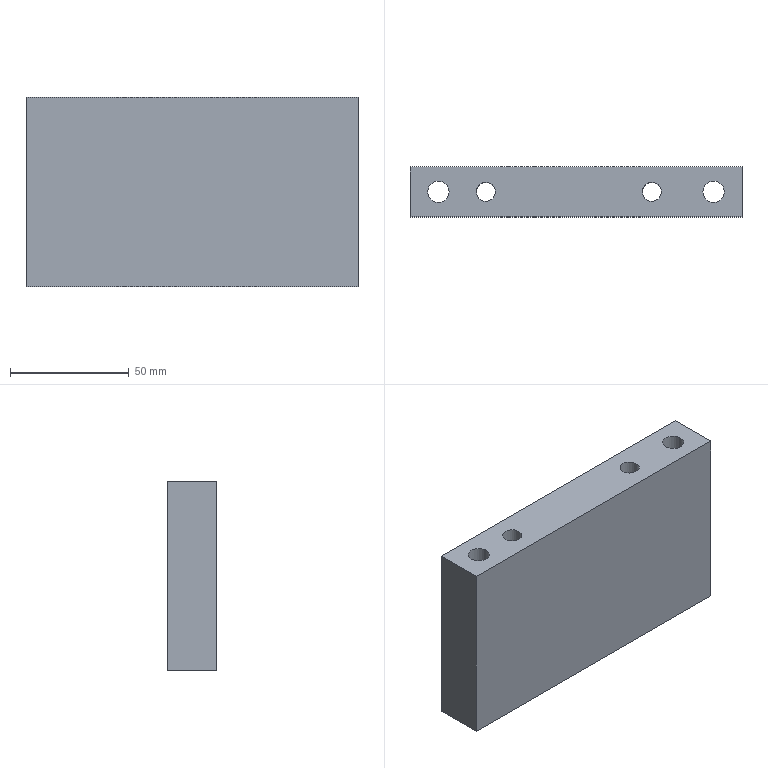Part | STEP file | lll_id3266_x_t | 1 solid | 16 faces | box 140 x 21 x 80 mm | volume 204597 mm3 | plane 8 | cylinder 7 | cone 1 | commonest cylinder face diameters 8 x2 9.009 x2 14.507 x2 6.805 x1
STEP:
#1=CARTESIAN_POINT('',(1612.,4.,2.5));
#2=VERTEX_POINT('',#1);
#3=CARTESIAN_POINT('',(1612.,0.00007614,2.5));
#4=DIRECTION('',(0.,0.,-1.));
#5=DIRECTION('',(0.,1.,0.));
#6=AXIS2_PLACEMENT_3D('',#3,#4,#5);
#7=CIRCLE('',#6,4.);
#8=EDGE_CURVE('',#2,#2,#7,.T.);
#9=ORIENTED_EDGE('',*,*,#8,.F.);
#10=EDGE_LOOP('',(#9));
#11=FACE_BOUND('',#10,.T.);
#12=CARTESIAN_POINT('',(1682.,4.,2.5));
#13=VERTEX_POINT('',#12);
#14=CARTESIAN_POINT('',(1682.,0.00007614,2.5));
#15=DIRECTION('',(0.,0.,-1.));
#16=DIRECTION('',(0.,1.,0.));
#17=AXIS2_PLACEMENT_3D('',#14,#15,#16);
#18=CIRCLE('',#17,4.);
#19=EDGE_CURVE('',#13,#13,#18,.T.);
#20=ORIENTED_EDGE('',*,*,#19,.F.);
#21=EDGE_LOOP('',(#20));
#22=FACE_BOUND('',#21,.T.);
#23=CARTESIAN_POINT('',(1670.402,0.00007614,2.5));
#24=VERTEX_POINT('',#23);
#25=CARTESIAN_POINT('',(1667.,0.00007614,2.5));
#26=DIRECTION('',(0.,0.,1.));
#27=DIRECTION('',(1.,0.,0.));
#28=AXIS2_PLACEMENT_3D('',#25,#26,#27);
#29=CIRCLE('',#28,3.402);
#30=EDGE_CURVE('',#24,#24,#29,.T.);
#31=ORIENTED_EDGE('',*,*,#30,.T.);
#32=EDGE_LOOP('',(#31));
#33=FACE_BOUND('',#32,.T.);
#34=CARTESIAN_POINT('',(1599.254,0.00007614,2.5));
#35=VERTEX_POINT('',#34);
#36=CARTESIAN_POINT('',(1592.,0.00007614,2.5));
#37=DIRECTION('',(0.,0.,1.));
#38=DIRECTION('',(1.,0.,0.));
#39=AXIS2_PLACEMENT_3D('',#36,#37,#38);
#40=CIRCLE('',#39,7.253);
#41=EDGE_CURVE('',#35,#35,#40,.T.);
#42=ORIENTED_EDGE('',*,*,#41,.T.);
#43=EDGE_LOOP('',(#42));
#44=FACE_BOUND('',#43,.T.);
#45=CARTESIAN_POINT('',(1580.,-10.5,2.5));
#46=VERTEX_POINT('',#45);
#47=CARTESIAN_POINT('',(1720.,-10.5,2.5));
#48=VERTEX_POINT('',#47);
#49=CARTESIAN_POINT('',(12283.883,-10.5,2.5));
#50=DIRECTION('',(1.,0.,0.));
#51=VECTOR('',#50,1.);
#52=LINE('',#49,#51);
#53=EDGE_CURVE('',#46,#48,#52,.T.);
#54=ORIENTED_EDGE('',*,*,#53,.F.);
#55=CARTESIAN_POINT('',(1580.,10.5,2.5));
#56=VERTEX_POINT('',#55);
#57=CARTESIAN_POINT('',(1580.,-13712.786,2.5));
#58=DIRECTION('',(0.,1.,0.));
#59=VECTOR('',#58,1.);
#60=LINE('',#57,#59);
#61=EDGE_CURVE('',#46,#56,#60,.T.);
#62=ORIENTED_EDGE('',*,*,#61,.T.);
#63=CARTESIAN_POINT('',(1720.,10.5,2.5));
#64=VERTEX_POINT('',#63);
#65=CARTESIAN_POINT('',(12283.883,10.5,2.5));
#66=DIRECTION('',(-1.,0.,0.));
#67=VECTOR('',#66,1.);
#68=LINE('',#65,#67);
#69=EDGE_CURVE('',#64,#56,#68,.T.);
#70=ORIENTED_EDGE('',*,*,#69,.F.);
#71=CARTESIAN_POINT('',(1720.,-13712.786,2.5));
#72=DIRECTION('',(0.,-1.,0.));
#73=VECTOR('',#72,1.);
#74=LINE('',#71,#73);
#75=EDGE_CURVE('',#64,#48,#74,.T.);
#76=ORIENTED_EDGE('',*,*,#75,.T.);
#77=EDGE_LOOP('',(#54,#62,#70,#76));
#78=FACE_BOUND('',#77,.T.);
#79=CARTESIAN_POINT('',(1715.254,0.00007614,2.5));
#80=VERTEX_POINT('',#79);
#81=CARTESIAN_POINT('',(1708.,0.00007614,2.5));
#82=DIRECTION('',(0.,0.,1.));
#83=DIRECTION('',(1.,0.,0.));
#84=AXIS2_PLACEMENT_3D('',#81,#82,#83);
#85=CIRCLE('',#84,7.253);
#86=EDGE_CURVE('',#80,#80,#85,.T.);
#87=ORIENTED_EDGE('',*,*,#86,.T.);
#88=EDGE_LOOP('',(#87));
#89=FACE_BOUND('',#88,.T.);
#90=CARTESIAN_POINT('',(12283.883,-13712.786,2.5));
#91=DIRECTION('',(0.,0.,-1.));
#92=DIRECTION('',(1.,0.,0.));
#93=AXIS2_PLACEMENT_3D('',#90,#91,#92);
#94=PLANE('',#93);
#95=ADVANCED_FACE('',(#11,#22,#33,#44,#78,#89),#94,.T.);
#96=ORIENTED_EDGE('',*,*,#53,.T.);
#97=CARTESIAN_POINT('',(1720.,-10.5,82.5));
#98=VERTEX_POINT('',#97);
#99=CARTESIAN_POINT('',(1720.,-10.5,50.));
#100=DIRECTION('',(0.,0.,-1.));
#101=VECTOR('',#100,1.);
#102=LINE('',#99,#101);
#103=EDGE_CURVE('',#98,#48,#102,.T.);
#104=ORIENTED_EDGE('',*,*,#103,.F.);
#105=CARTESIAN_POINT('',(1580.,-10.5,82.5));
#106=VERTEX_POINT('',#105);
#107=CARTESIAN_POINT('',(2347.435,-10.5,82.5));
#108=DIRECTION('',(1.,0.,0.));
#109=VECTOR('',#108,1.);
#110=LINE('',#107,#109);
#111=EDGE_CURVE('',#106,#98,#110,.T.);
#112=ORIENTED_EDGE('',*,*,#111,.F.);
#113=CARTESIAN_POINT('',(1580.,-10.5,50.));
#114=DIRECTION('',(0.,0.,-1.));
#115=VECTOR('',#114,1.);
#116=LINE('',#113,#115);
#117=EDGE_CURVE('',#106,#46,#116,.T.);
#118=ORIENTED_EDGE('',*,*,#117,.T.);
#119=EDGE_LOOP('',(#96,#104,#112,#118));
#120=FACE_OUTER_BOUND('',#119,.T.);
#121=CARTESIAN_POINT('',(1590.,-10.5,50.));
#122=DIRECTION('',(0.,1.,0.));
#123=DIRECTION('',(0.,0.,1.));
#124=AXIS2_PLACEMENT_3D('',#121,#122,#123);
#125=PLANE('',#124);
#126=ADVANCED_FACE('',(#120),#125,.F.);
#127=ORIENTED_EDGE('',*,*,#75,.F.);
#128=CARTESIAN_POINT('',(1720.,10.5,82.5));
#129=VERTEX_POINT('',#128);
#130=CARTESIAN_POINT('',(1720.,10.5,50.));
#131=DIRECTION('',(0.,0.,-1.));
#132=VECTOR('',#131,1.);
#133=LINE('',#130,#132);
#134=EDGE_CURVE('',#129,#64,#133,.T.);
#135=ORIENTED_EDGE('',*,*,#134,.F.);
#136=CARTESIAN_POINT('',(1720.,0.,82.5));
#137=DIRECTION('',(0.,-1.,0.));
#138=VECTOR('',#137,1.);
#139=LINE('',#136,#138);
#140=EDGE_CURVE('',#129,#98,#139,.T.);
#141=ORIENTED_EDGE('',*,*,#140,.T.);
#142=ORIENTED_EDGE('',*,*,#103,.T.);
#143=EDGE_LOOP('',(#127,#135,#141,#142));
#144=FACE_OUTER_BOUND('',#143,.T.);
#145=CARTESIAN_POINT('',(1720.,7.5,50.));
#146=DIRECTION('',(1.,0.,0.));
#147=DIRECTION('',(0.,0.,-1.));
#148=AXIS2_PLACEMENT_3D('',#145,#146,#147);
#149=PLANE('',#148);
#150=ADVANCED_FACE('',(#144),#149,.T.);
#151=ORIENTED_EDGE('',*,*,#69,.T.);
#152=CARTESIAN_POINT('',(1580.,10.5,82.5));
#153=VERTEX_POINT('',#152);
#154=CARTESIAN_POINT('',(1580.,10.5,50.));
#155=DIRECTION('',(0.,0.,-1.));
#156=VECTOR('',#155,1.);
#157=LINE('',#154,#156);
#158=EDGE_CURVE('',#153,#56,#157,.T.);
#159=ORIENTED_EDGE('',*,*,#158,.F.);
#160=CARTESIAN_POINT('',(2347.435,10.5,82.5));
#161=DIRECTION('',(-1.,0.,0.));
#162=VECTOR('',#161,1.);
#163=LINE('',#160,#162);
#164=EDGE_CURVE('',#129,#153,#163,.T.);
#165=ORIENTED_EDGE('',*,*,#164,.F.);
#166=ORIENTED_EDGE('',*,*,#134,.T.);
#167=EDGE_LOOP('',(#151,#159,#165,#166));
#168=FACE_OUTER_BOUND('',#167,.T.);
#169=CARTESIAN_POINT('',(1660.,10.5,50.));
#170=DIRECTION('',(0.,-1.,0.));
#171=DIRECTION('',(0.,0.,-1.));
#172=AXIS2_PLACEMENT_3D('',#169,#170,#171);
#173=PLANE('',#172);
#174=ADVANCED_FACE('',(#168),#173,.F.);
#175=ORIENTED_EDGE('',*,*,#61,.F.);
#176=ORIENTED_EDGE('',*,*,#117,.F.);
#177=CARTESIAN_POINT('',(1580.,0.,82.5));
#178=DIRECTION('',(0.,1.,0.));
#179=VECTOR('',#178,1.);
#180=LINE('',#177,#179);
#181=EDGE_CURVE('',#106,#153,#180,.T.);
#182=ORIENTED_EDGE('',*,*,#181,.T.);
#183=ORIENTED_EDGE('',*,*,#158,.T.);
#184=EDGE_LOOP('',(#175,#176,#182,#183));
#185=FACE_OUTER_BOUND('',#184,.T.);
#186=CARTESIAN_POINT('',(1580.,-7.5,50.));
#187=DIRECTION('',(-1.,0.,0.));
#188=DIRECTION('',(0.,0.,1.));
#189=AXIS2_PLACEMENT_3D('',#186,#187,#188);
#190=PLANE('',#189);
#191=ADVANCED_FACE('',(#185),#190,.T.);
#192=CARTESIAN_POINT('',(1678.,0.00007614,82.5));
#193=VERTEX_POINT('',#192);
#194=CARTESIAN_POINT('',(1682.,0.00007614,82.5));
#195=DIRECTION('',(0.,0.,-1.));
#196=DIRECTION('',(-1.,0.,0.));
#197=AXIS2_PLACEMENT_3D('',#194,#195,#196);
#198=CIRCLE('',#197,4.);
#199=EDGE_CURVE('',#193,#193,#198,.T.);
#200=ORIENTED_EDGE('',*,*,#199,.T.);
#201=EDGE_LOOP('',(#200));
#202=FACE_BOUND('',#201,.T.);
#203=CARTESIAN_POINT('',(1608.,0.00007614,82.5));
#204=VERTEX_POINT('',#203);
#205=CARTESIAN_POINT('',(1612.,0.00007614,82.5));
#206=DIRECTION('',(0.,0.,-1.));
#207=DIRECTION('',(-1.,0.,0.));
#208=AXIS2_PLACEMENT_3D('',#205,#206,#207);
#209=CIRCLE('',#208,4.);
#210=EDGE_CURVE('',#204,#204,#209,.T.);
#211=ORIENTED_EDGE('',*,*,#210,.T.);
#212=EDGE_LOOP('',(#211));
#213=FACE_BOUND('',#212,.T.);
#214=CARTESIAN_POINT('',(1703.495,0.00007614,82.5));
#215=VERTEX_POINT('',#214);
#216=CARTESIAN_POINT('',(1708.,0.00007614,82.5));
#217=DIRECTION('',(0.,0.,-1.));
#218=DIRECTION('',(-1.,0.,0.));
#219=AXIS2_PLACEMENT_3D('',#216,#217,#218);
#220=CIRCLE('',#219,4.505);
#221=EDGE_CURVE('',#215,#215,#220,.T.);
#222=ORIENTED_EDGE('',*,*,#221,.T.);
#223=EDGE_LOOP('',(#222));
#224=FACE_BOUND('',#223,.T.);
#225=CARTESIAN_POINT('',(1587.495,0.00007614,82.5));
#226=VERTEX_POINT('',#225);
#227=CARTESIAN_POINT('',(1592.,0.00007614,82.5));
#228=DIRECTION('',(0.,0.,-1.));
#229=DIRECTION('',(-1.,0.,0.));
#230=AXIS2_PLACEMENT_3D('',#227,#228,#229);
#231=CIRCLE('',#230,4.505);
#232=EDGE_CURVE('',#226,#226,#231,.T.);
#233=ORIENTED_EDGE('',*,*,#232,.T.);
#234=EDGE_LOOP('',(#233));
#235=FACE_BOUND('',#234,.T.);
#236=ORIENTED_EDGE('',*,*,#111,.T.);
#237=ORIENTED_EDGE('',*,*,#140,.F.);
#238=ORIENTED_EDGE('',*,*,#164,.T.);
#239=ORIENTED_EDGE('',*,*,#181,.F.);
#240=EDGE_LOOP('',(#236,#237,#238,#239));
#241=FACE_BOUND('',#240,.T.);
#242=CARTESIAN_POINT('',(2347.435,0.,82.5));
#243=DIRECTION('',(0.,0.,-1.));
#244=DIRECTION('',(1.,0.,0.));
#245=AXIS2_PLACEMENT_3D('',#242,#243,#244);
#246=PLANE('',#245);
#247=ADVANCED_FACE('',(#202,#213,#224,#235,#241),#246,.F.);
#248=CARTESIAN_POINT('',(1596.505,0.00007614,57.5));
#249=VERTEX_POINT('',#248);
#250=CARTESIAN_POINT('',(1592.,0.00007614,57.5));
#251=DIRECTION('',(0.,0.,1.));
#252=DIRECTION('',(1.,0.,0.));
#253=AXIS2_PLACEMENT_3D('',#250,#251,#252);
#254=CIRCLE('',#253,4.505);
#255=EDGE_CURVE('',#249,#249,#254,.T.);
#256=ORIENTED_EDGE('',*,*,#255,.F.);
#257=EDGE_LOOP('',(#256));
#258=FACE_BOUND('',#257,.T.);
#259=ORIENTED_EDGE('',*,*,#232,.F.);
#260=EDGE_LOOP('',(#259));
#261=FACE_BOUND('',#260,.T.);
#262=CARTESIAN_POINT('',(1592.,0.00007614,-2.5));
#263=DIRECTION('',(0.,0.,1.));
#264=DIRECTION('',(1.,0.,0.));
#265=AXIS2_PLACEMENT_3D('',#262,#263,#264);
#266=CYLINDRICAL_SURFACE('',#265,4.505);
#267=ADVANCED_FACE('',(#258,#261),#266,.F.);
#268=ORIENTED_EDGE('',*,*,#255,.T.);
#269=EDGE_LOOP('',(#268));
#270=FACE_BOUND('',#269,.T.);
#271=CARTESIAN_POINT('',(1599.254,0.00007614,57.5));
#272=VERTEX_POINT('',#271);
#273=CARTESIAN_POINT('',(1592.,0.00007614,57.5));
#274=DIRECTION('',(0.,0.,1.));
#275=DIRECTION('',(1.,0.,0.));
#276=AXIS2_PLACEMENT_3D('',#273,#274,#275);
#277=CIRCLE('',#276,7.253);
#278=EDGE_CURVE('',#272,#272,#277,.T.);
#279=ORIENTED_EDGE('',*,*,#278,.F.);
#280=EDGE_LOOP('',(#279));
#281=FACE_BOUND('',#280,.T.);
#282=CARTESIAN_POINT('',(1592.,0.00007614,57.5));
#283=DIRECTION('',(0.,0.,1.));
#284=DIRECTION('',(1.,0.,0.));
#285=AXIS2_PLACEMENT_3D('',#282,#283,#284);
#286=PLANE('',#285);
#287=ADVANCED_FACE('',(#270,#281),#286,.F.);
#288=ORIENTED_EDGE('',*,*,#278,.T.);
#289=EDGE_LOOP('',(#288));
#290=FACE_BOUND('',#289,.T.);
#291=ORIENTED_EDGE('',*,*,#41,.F.);
#292=EDGE_LOOP('',(#291));
#293=FACE_BOUND('',#292,.T.);
#294=CARTESIAN_POINT('',(1592.,0.00007614,2.5));
#295=DIRECTION('',(0.,0.,1.));
#296=DIRECTION('',(1.,0.,0.));
#297=AXIS2_PLACEMENT_3D('',#294,#295,#296);
#298=CYLINDRICAL_SURFACE('',#297,7.253);
#299=ADVANCED_FACE('',(#290,#293),#298,.F.);
#300=CARTESIAN_POINT('',(1712.505,0.00007614,57.5));
#301=VERTEX_POINT('',#300);
#302=CARTESIAN_POINT('',(1708.,0.00007614,57.5));
#303=DIRECTION('',(0.,0.,1.));
#304=DIRECTION('',(1.,0.,0.));
#305=AXIS2_PLACEMENT_3D('',#302,#303,#304);
#306=CIRCLE('',#305,4.505);
#307=EDGE_CURVE('',#301,#301,#306,.T.);
#308=ORIENTED_EDGE('',*,*,#307,.F.);
#309=EDGE_LOOP('',(#308));
#310=FACE_BOUND('',#309,.T.);
#311=ORIENTED_EDGE('',*,*,#221,.F.);
#312=EDGE_LOOP('',(#311));
#313=FACE_BOUND('',#312,.T.);
#314=CARTESIAN_POINT('',(1708.,0.00007614,-2.5));
#315=DIRECTION('',(0.,0.,1.));
#316=DIRECTION('',(1.,0.,0.));
#317=AXIS2_PLACEMENT_3D('',#314,#315,#316);
#318=CYLINDRICAL_SURFACE('',#317,4.505);
#319=ADVANCED_FACE('',(#310,#313),#318,.F.);
#320=ORIENTED_EDGE('',*,*,#307,.T.);
#321=EDGE_LOOP('',(#320));
#322=FACE_BOUND('',#321,.T.);
#323=CARTESIAN_POINT('',(1715.254,0.00007614,57.5));
#324=VERTEX_POINT('',#323);
#325=CARTESIAN_POINT('',(1708.,0.00007614,57.5));
#326=DIRECTION('',(0.,0.,1.));
#327=DIRECTION('',(1.,0.,0.));
#328=AXIS2_PLACEMENT_3D('',#325,#326,#327);
#329=CIRCLE('',#328,7.253);
#330=EDGE_CURVE('',#324,#324,#329,.T.);
#331=ORIENTED_EDGE('',*,*,#330,.F.);
#332=EDGE_LOOP('',(#331));
#333=FACE_BOUND('',#332,.T.);
#334=CARTESIAN_POINT('',(1708.,0.00007614,57.5));
#335=DIRECTION('',(0.,0.,1.));
#336=DIRECTION('',(1.,0.,0.));
#337=AXIS2_PLACEMENT_3D('',#334,#335,#336);
#338=PLANE('',#337);
#339=ADVANCED_FACE('',(#322,#333),#338,.F.);
#340=ORIENTED_EDGE('',*,*,#330,.T.);
#341=EDGE_LOOP('',(#340));
#342=FACE_BOUND('',#341,.T.);
#343=ORIENTED_EDGE('',*,*,#86,.F.);
#344=EDGE_LOOP('',(#343));
#345=FACE_BOUND('',#344,.T.);
#346=CARTESIAN_POINT('',(1708.,0.00007614,2.5));
#347=DIRECTION('',(0.,0.,1.));
#348=DIRECTION('',(1.,0.,0.));
#349=AXIS2_PLACEMENT_3D('',#346,#347,#348);
#350=CYLINDRICAL_SURFACE('',#349,7.253);
#351=ADVANCED_FACE('',(#342,#345),#350,.F.);
#352=ORIENTED_EDGE('',*,*,#210,.F.);
#353=EDGE_LOOP('',(#352));
#354=FACE_BOUND('',#353,.T.);
#355=ORIENTED_EDGE('',*,*,#8,.T.);
#356=EDGE_LOOP('',(#355));
#357=FACE_BOUND('',#356,.T.);
#358=CARTESIAN_POINT('',(1612.,0.00007614,2.5));
#359=DIRECTION('',(0.,0.,1.));
#360=DIRECTION('',(1.,0.,0.));
#361=AXIS2_PLACEMENT_3D('',#358,#359,#360);
#362=CYLINDRICAL_SURFACE('',#361,4.);
#363=ADVANCED_FACE('',(#354,#357),#362,.F.);
#364=CARTESIAN_POINT('',(1667.,-3.402,34.103));
#365=VERTEX_POINT('',#364);
#366=CARTESIAN_POINT('',(1667.,0.00007614,34.103));
#367=DIRECTION('',(0.,0.,1.));
#368=DIRECTION('',(0.,-1.,0.));
#369=AXIS2_PLACEMENT_3D('',#366,#367,#368);
#370=CIRCLE('',#369,3.402);
#371=EDGE_CURVE('',#365,#365,#370,.T.);
#372=ORIENTED_EDGE('',*,*,#371,.T.);
#373=EDGE_LOOP('',(#372));
#374=FACE_BOUND('',#373,.T.);
#375=ORIENTED_EDGE('',*,*,#30,.F.);
#376=EDGE_LOOP('',(#375));
#377=FACE_BOUND('',#376,.T.);
#378=CARTESIAN_POINT('',(1667.,0.00007614,2.5));
#379=DIRECTION('',(0.,0.,1.));
#380=DIRECTION('',(1.,0.,0.));
#381=AXIS2_PLACEMENT_3D('',#378,#379,#380);
#382=CYLINDRICAL_SURFACE('',#381,3.402);
#383=ADVANCED_FACE('',(#374,#377),#382,.F.);
#384=CARTESIAN_POINT('',(1667.,0.00007614,37.506));
#385=VERTEX_POINT('',#384);
#386=VERTEX_LOOP('',#385);
#387=FACE_BOUND('',#386,.T.);
#388=ORIENTED_EDGE('',*,*,#371,.F.);
#389=EDGE_LOOP('',(#388));
#390=FACE_BOUND('',#389,.T.);
#391=CARTESIAN_POINT('',(1667.,0.00007614,34.103));
#392=DIRECTION('',(0.,0.,-1.));
#393=DIRECTION('',(0.,1.,0.));
#394=AXIS2_PLACEMENT_3D('',#391,#392,#393);
#395=CONICAL_SURFACE('',#394,3.402,45.);
#396=ADVANCED_FACE('',(#387,#390),#395,.F.);
#397=ORIENTED_EDGE('',*,*,#199,.F.);
#398=EDGE_LOOP('',(#397));
#399=FACE_BOUND('',#398,.T.);
#400=ORIENTED_EDGE('',*,*,#19,.T.);
#401=EDGE_LOOP('',(#400));
#402=FACE_BOUND('',#401,.T.);
#403=CARTESIAN_POINT('',(1682.,0.00007614,2.5));
#404=DIRECTION('',(0.,0.,1.));
#405=DIRECTION('',(1.,0.,0.));
#406=AXIS2_PLACEMENT_3D('',#403,#404,#405);
#407=CYLINDRICAL_SURFACE('',#406,4.);
#408=ADVANCED_FACE('',(#399,#402),#407,.F.);
#409=CLOSED_SHELL('',(#95,#126,#150,#174,#191,#247,#267,#287,#299,#319,#339,#351,#363,#383,#396,#408));
#410=MANIFOLD_SOLID_BREP('',#409);
#411=(LENGTH_UNIT()NAMED_UNIT(*)SI_UNIT(.MILLI.,.METRE.));
#412=UNCERTAINTY_MEASURE_WITH_UNIT(LENGTH_MEASURE(0.00002),#411,'','');
#413=(NAMED_UNIT(*)PLANE_ANGLE_UNIT()SI_UNIT($,.RADIAN.));
#414=PLANE_ANGLE_MEASURE_WITH_UNIT(PLANE_ANGLE_MEASURE(0.01745),#413);
#415=DIMENSIONAL_EXPONENTS(0.,0.,0.,0.,0.,0.,0.);
#416=(CONVERSION_BASED_UNIT('DEGREE',#414)NAMED_UNIT(#415)PLANE_ANGLE_UNIT());
#417=(NAMED_UNIT(*)SI_UNIT($,.STERADIAN.)SOLID_ANGLE_UNIT());
#418=(GEOMETRIC_REPRESENTATION_CONTEXT(3)GLOBAL_UNCERTAINTY_ASSIGNED_CONTEXT((#412))GLOBAL_UNIT_ASSIGNED_CONTEXT((#411,#416,#417))REPRESENTATION_CONTEXT('',''));
#419=ADVANCED_BREP_SHAPE_REPRESENTATION('',(#410),#418);